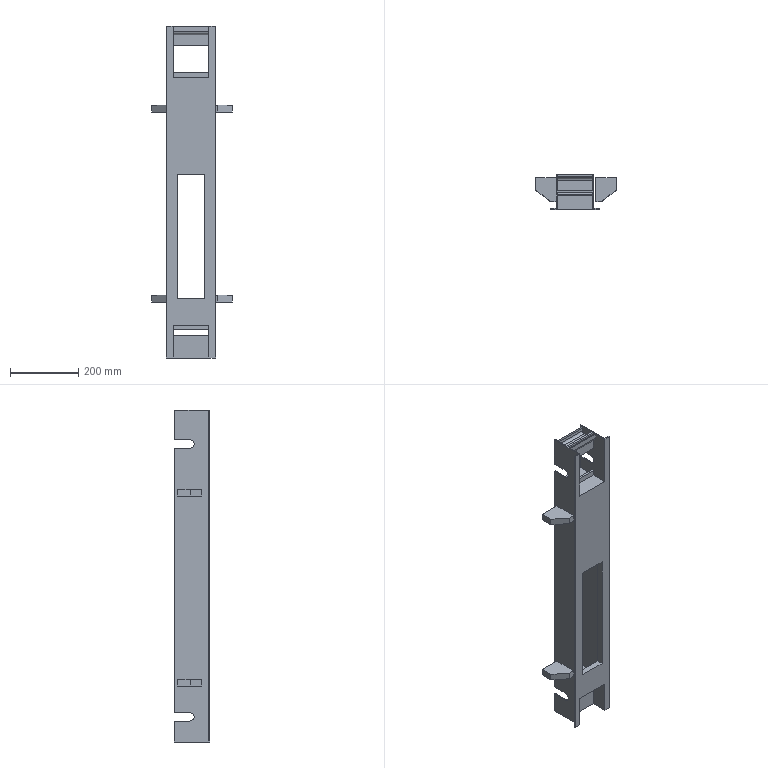Part | STEP file | 3 solids | 102 faces | box 236 x 103 x 974 mm | volume 2291572 mm3 | plane 95 | cylinder 7 | commonest cylinder face diameters 25 x3 14 x2 20 x2